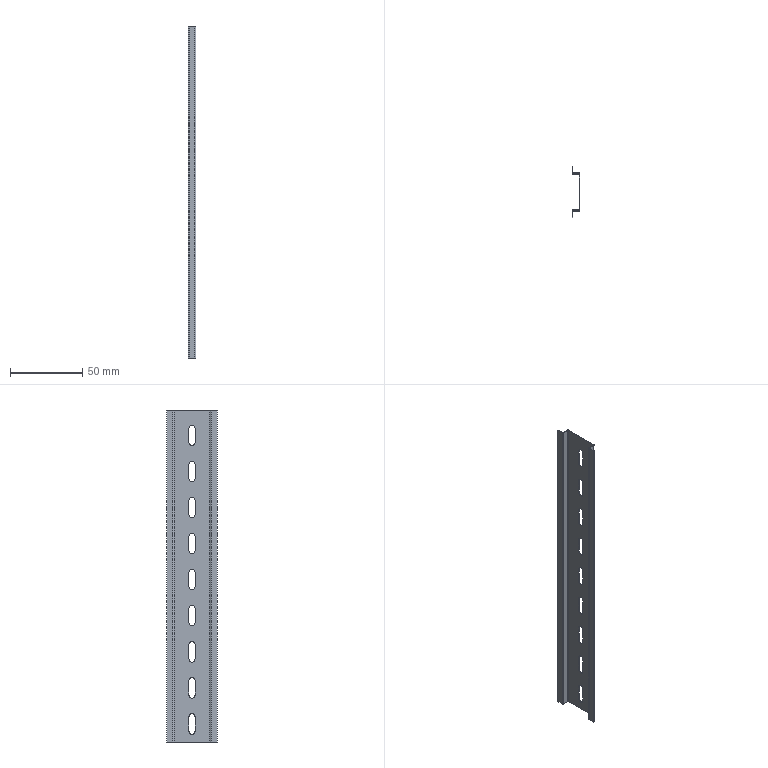Part | STEP file | 1 solid | 74 faces | box 5.5 x 35 x 230 mm | volume 4835 mm3 | plane 48 | cylinder 26 | commonest cylinder face diameters 4.2 x18 0.4 x4 1.4 x4